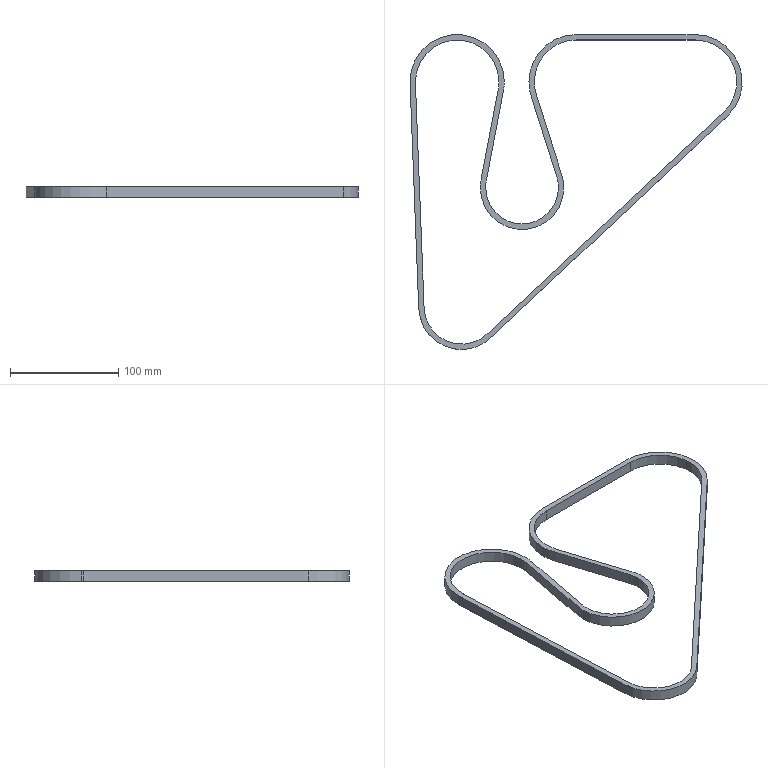Part | SolidWorks | features BeltProfileFeature 1, ExtruThin 1 | 1 solid | 32 faces | box 307.239 x 291.218 x 10 mm | volume 65563 mm3 | cylinder 20 | plane 12 | commonest cylinder face diameters 77.239 x9 87.239 x6 67.239 x3 69.196 x1 79.196 x1
STEP:
#1=CARTESIAN_POINT('',(33.941,200.791,10.));
#2=VERTEX_POINT('',#1);
#3=CARTESIAN_POINT('',(34.62,208.,10.));
#4=VERTEX_POINT('',#3);
#5=CARTESIAN_POINT('',(-4.,208.,10.));
#6=DIRECTION('',(0.,0.,1.));
#7=DIRECTION('',(-1.,0.,0.));
#8=AXIS2_PLACEMENT_3D('',#5,#6,#7);
#9=CIRCLE('',#8,38.62);
#10=EDGE_CURVE('',#2,#4,#9,.T.);
#11=ORIENTED_EDGE('',*,*,#10,.T.);
#12=CARTESIAN_POINT('',(34.62,208.,0.));
#13=VERTEX_POINT('',#12);
#14=CARTESIAN_POINT('',(34.62,208.,10.));
#15=DIRECTION('',(0.,0.,-1.));
#16=VECTOR('',#15,1000.);
#17=LINE('',#14,#16);
#18=EDGE_CURVE('',#4,#13,#17,.T.);
#19=ORIENTED_EDGE('',*,*,#18,.T.);
#20=CARTESIAN_POINT('',(33.941,200.791,0.));
#21=VERTEX_POINT('',#20);
#22=CARTESIAN_POINT('',(-4.,208.,0.));
#23=DIRECTION('',(0.,0.,1.));
#24=DIRECTION('',(-1.,0.,0.));
#25=AXIS2_PLACEMENT_3D('',#22,#23,#24);
#26=CIRCLE('',#25,38.62);
#27=EDGE_CURVE('',#21,#13,#26,.T.);
#28=ORIENTED_EDGE('',*,*,#27,.F.);
#29=CARTESIAN_POINT('',(33.941,200.791,10.));
#30=DIRECTION('',(0.,0.,-1.));
#31=VECTOR('',#30,1000.);
#32=LINE('',#29,#31);
#33=EDGE_CURVE('',#2,#21,#32,.T.);
#34=ORIENTED_EDGE('',*,*,#33,.F.);
#35=EDGE_LOOP('',(#11,#19,#28,#34));
#36=FACE_OUTER_BOUND('',#35,.T.);
#37=CARTESIAN_POINT('',(-4.,208.,10.));
#38=DIRECTION('',(0.,0.,-1.));
#39=DIRECTION('',(-1.,0.,0.));
#40=AXIS2_PLACEMENT_3D('',#37,#38,#39);
#41=CYLINDRICAL_SURFACE('',#40,38.62);
#42=ADVANCED_FACE('',(#36),#41,.F.);
#43=ORIENTED_EDGE('',*,*,#18,.F.);
#44=CARTESIAN_POINT('',(-42.62,208.,10.));
#45=VERTEX_POINT('',#44);
#46=CARTESIAN_POINT('',(-4.,208.,10.));
#47=DIRECTION('',(0.,0.,1.));
#48=DIRECTION('',(-1.,0.,0.));
#49=AXIS2_PLACEMENT_3D('',#46,#47,#48);
#50=CIRCLE('',#49,38.62);
#51=EDGE_CURVE('',#4,#45,#50,.T.);
#52=ORIENTED_EDGE('',*,*,#51,.T.);
#53=CARTESIAN_POINT('',(-42.62,208.,0.));
#54=VERTEX_POINT('',#53);
#55=CARTESIAN_POINT('',(-42.62,208.,10.));
#56=DIRECTION('',(0.,0.,-1.));
#57=VECTOR('',#56,1000.);
#58=LINE('',#55,#57);
#59=EDGE_CURVE('',#45,#54,#58,.T.);
#60=ORIENTED_EDGE('',*,*,#59,.T.);
#61=CARTESIAN_POINT('',(-4.,208.,0.));
#62=DIRECTION('',(0.,0.,1.));
#63=DIRECTION('',(-1.,0.,0.));
#64=AXIS2_PLACEMENT_3D('',#61,#62,#63);
#65=CIRCLE('',#64,38.62);
#66=EDGE_CURVE('',#13,#54,#65,.T.);
#67=ORIENTED_EDGE('',*,*,#66,.F.);
#68=EDGE_LOOP('',(#43,#52,#60,#67));
#69=FACE_OUTER_BOUND('',#68,.T.);
#70=CARTESIAN_POINT('',(-4.,208.,10.));
#71=DIRECTION('',(0.,0.,-1.));
#72=DIRECTION('',(-1.,0.,0.));
#73=AXIS2_PLACEMENT_3D('',#70,#71,#72);
#74=CYLINDRICAL_SURFACE('',#73,38.62);
#75=ADVANCED_FACE('',(#69),#74,.F.);
#76=CARTESIAN_POINT('',(92.82,121.653,10.));
#77=VERTEX_POINT('',#76);
#78=CARTESIAN_POINT('',(94.62,110.,10.));
#79=VERTEX_POINT('',#78);
#80=CARTESIAN_POINT('',(56.,110.,10.));
#81=DIRECTION('',(0.,0.,-1.));
#82=DIRECTION('',(1.,0.,0.));
#83=AXIS2_PLACEMENT_3D('',#80,#81,#82);
#84=CIRCLE('',#83,38.62);
#85=EDGE_CURVE('',#77,#79,#84,.T.);
#86=ORIENTED_EDGE('',*,*,#85,.T.);
#87=CARTESIAN_POINT('',(94.62,110.,0.));
#88=VERTEX_POINT('',#87);
#89=CARTESIAN_POINT('',(94.62,110.,10.));
#90=DIRECTION('',(0.,0.,-1.));
#91=VECTOR('',#90,1000.);
#92=LINE('',#89,#91);
#93=EDGE_CURVE('',#79,#88,#92,.T.);
#94=ORIENTED_EDGE('',*,*,#93,.T.);
#95=CARTESIAN_POINT('',(92.82,121.653,0.));
#96=VERTEX_POINT('',#95);
#97=CARTESIAN_POINT('',(56.,110.,0.));
#98=DIRECTION('',(0.,0.,-1.));
#99=DIRECTION('',(1.,0.,0.));
#100=AXIS2_PLACEMENT_3D('',#97,#98,#99);
#101=CIRCLE('',#100,38.62);
#102=EDGE_CURVE('',#96,#88,#101,.T.);
#103=ORIENTED_EDGE('',*,*,#102,.F.);
#104=CARTESIAN_POINT('',(92.82,121.653,10.));
#105=DIRECTION('',(0.,0.,-1.));
#106=VECTOR('',#105,1000.);
#107=LINE('',#104,#106);
#108=EDGE_CURVE('',#77,#96,#107,.T.);
#109=ORIENTED_EDGE('',*,*,#108,.F.);
#110=EDGE_LOOP('',(#86,#94,#103,#109));
#111=FACE_OUTER_BOUND('',#110,.T.);
#112=CARTESIAN_POINT('',(56.,110.,10.));
#113=DIRECTION('',(0.,0.,-1.));
#114=DIRECTION('',(-1.,0.,0.));
#115=AXIS2_PLACEMENT_3D('',#112,#113,#114);
#116=CYLINDRICAL_SURFACE('',#115,38.62);
#117=ADVANCED_FACE('',(#111),#116,.T.);
#118=ORIENTED_EDGE('',*,*,#93,.F.);
#119=CARTESIAN_POINT('',(17.38,110.,10.));
#120=VERTEX_POINT('',#119);
#121=CARTESIAN_POINT('',(56.,110.,10.));
#122=DIRECTION('',(0.,0.,-1.));
#123=DIRECTION('',(1.,0.,0.));
#124=AXIS2_PLACEMENT_3D('',#121,#122,#123);
#125=CIRCLE('',#124,38.62);
#126=EDGE_CURVE('',#79,#120,#125,.T.);
#127=ORIENTED_EDGE('',*,*,#126,.T.);
#128=CARTESIAN_POINT('',(17.38,110.,0.));
#129=VERTEX_POINT('',#128);
#130=CARTESIAN_POINT('',(17.38,110.,10.));
#131=DIRECTION('',(0.,0.,-1.));
#132=VECTOR('',#131,1000.);
#133=LINE('',#130,#132);
#134=EDGE_CURVE('',#120,#129,#133,.T.);
#135=ORIENTED_EDGE('',*,*,#134,.T.);
#136=CARTESIAN_POINT('',(56.,110.,0.));
#137=DIRECTION('',(0.,0.,-1.));
#138=DIRECTION('',(1.,0.,0.));
#139=AXIS2_PLACEMENT_3D('',#136,#137,#138);
#140=CIRCLE('',#139,38.62);
#141=EDGE_CURVE('',#88,#129,#140,.T.);
#142=ORIENTED_EDGE('',*,*,#141,.F.);
#143=EDGE_LOOP('',(#118,#127,#135,#142));
#144=FACE_OUTER_BOUND('',#143,.T.);
#145=CARTESIAN_POINT('',(56.,110.,10.));
#146=DIRECTION('',(0.,0.,-1.));
#147=DIRECTION('',(-1.,0.,0.));
#148=AXIS2_PLACEMENT_3D('',#145,#146,#147);
#149=CYLINDRICAL_SURFACE('',#148,38.62);
#150=ADVANCED_FACE('',(#144),#149,.T.);
#151=CARTESIAN_POINT('',(106.,246.62,10.));
#152=VERTEX_POINT('',#151);
#153=CARTESIAN_POINT('',(67.38,208.,10.));
#154=VERTEX_POINT('',#153);
#155=CARTESIAN_POINT('',(106.,208.,10.));
#156=DIRECTION('',(0.,0.,1.));
#157=DIRECTION('',(-1.,0.,0.));
#158=AXIS2_PLACEMENT_3D('',#155,#156,#157);
#159=CIRCLE('',#158,38.62);
#160=EDGE_CURVE('',#152,#154,#159,.T.);
#161=ORIENTED_EDGE('',*,*,#160,.T.);
#162=CARTESIAN_POINT('',(67.38,208.,0.));
#163=VERTEX_POINT('',#162);
#164=CARTESIAN_POINT('',(67.38,208.,10.));
#165=DIRECTION('',(0.,0.,-1.));
#166=VECTOR('',#165,1000.);
#167=LINE('',#164,#166);
#168=EDGE_CURVE('',#154,#163,#167,.T.);
#169=ORIENTED_EDGE('',*,*,#168,.T.);
#170=CARTESIAN_POINT('',(106.,246.62,0.));
#171=VERTEX_POINT('',#170);
#172=CARTESIAN_POINT('',(106.,208.,0.));
#173=DIRECTION('',(0.,0.,1.));
#174=DIRECTION('',(-1.,0.,0.));
#175=AXIS2_PLACEMENT_3D('',#172,#173,#174);
#176=CIRCLE('',#175,38.62);
#177=EDGE_CURVE('',#171,#163,#176,.T.);
#178=ORIENTED_EDGE('',*,*,#177,.F.);
#179=CARTESIAN_POINT('',(106.,246.62,10.));
#180=DIRECTION('',(0.,0.,-1.));
#181=VECTOR('',#180,1000.);
#182=LINE('',#179,#181);
#183=EDGE_CURVE('',#152,#171,#182,.T.);
#184=ORIENTED_EDGE('',*,*,#183,.F.);
#185=EDGE_LOOP('',(#161,#169,#178,#184));
#186=FACE_OUTER_BOUND('',#185,.T.);
#187=CARTESIAN_POINT('',(106.,208.,10.));
#188=DIRECTION('',(0.,0.,-1.));
#189=DIRECTION('',(-1.,0.,0.));
#190=AXIS2_PLACEMENT_3D('',#187,#188,#189);
#191=CYLINDRICAL_SURFACE('',#190,38.62);
#192=ADVANCED_FACE('',(#186),#191,.F.);
#193=CARTESIAN_POINT('',(39.62,208.,10.));
#194=VERTEX_POINT('',#193);
#195=CARTESIAN_POINT('',(-47.62,208.,10.));
#196=VERTEX_POINT('',#195);
#197=CARTESIAN_POINT('',(-4.,208.,10.));
#198=DIRECTION('',(0.,0.,1.));
#199=DIRECTION('',(-1.,0.,0.));
#200=AXIS2_PLACEMENT_3D('',#197,#198,#199);
#201=CIRCLE('',#200,43.62);
#202=EDGE_CURVE('',#194,#196,#201,.T.);
#203=ORIENTED_EDGE('',*,*,#202,.F.);
#204=CARTESIAN_POINT('',(39.62,208.,0.));
#205=VERTEX_POINT('',#204);
#206=CARTESIAN_POINT('',(39.62,208.,10.));
#207=DIRECTION('',(0.,0.,-1.));
#208=VECTOR('',#207,1000.);
#209=LINE('',#206,#208);
#210=EDGE_CURVE('',#194,#205,#209,.T.);
#211=ORIENTED_EDGE('',*,*,#210,.T.);
#212=CARTESIAN_POINT('',(-47.62,208.,0.));
#213=VERTEX_POINT('',#212);
#214=CARTESIAN_POINT('',(-4.,208.,0.));
#215=DIRECTION('',(0.,0.,1.));
#216=DIRECTION('',(-1.,0.,0.));
#217=AXIS2_PLACEMENT_3D('',#214,#215,#216);
#218=CIRCLE('',#217,43.62);
#219=EDGE_CURVE('',#205,#213,#218,.T.);
#220=ORIENTED_EDGE('',*,*,#219,.T.);
#221=CARTESIAN_POINT('',(-47.62,208.,10.));
#222=DIRECTION('',(0.,0.,-1.));
#223=VECTOR('',#222,1000.);
#224=LINE('',#221,#223);
#225=EDGE_CURVE('',#196,#213,#224,.T.);
#226=ORIENTED_EDGE('',*,*,#225,.F.);
#227=EDGE_LOOP('',(#203,#211,#220,#226));
#228=FACE_OUTER_BOUND('',#227,.T.);
#229=CARTESIAN_POINT('',(-4.,208.,10.));
#230=DIRECTION('',(0.,0.,-1.));
#231=DIRECTION('',(-1.,0.,0.));
#232=AXIS2_PLACEMENT_3D('',#229,#230,#231);
#233=CYLINDRICAL_SURFACE('',#232,43.62);
#234=ADVANCED_FACE('',(#228),#233,.T.);
#235=CARTESIAN_POINT('',(-47.587,206.318,10.));
#236=VERTEX_POINT('',#235);
#237=CARTESIAN_POINT('',(-4.,208.,10.));
#238=DIRECTION('',(0.,0.,1.));
#239=DIRECTION('',(-1.,0.,0.));
#240=AXIS2_PLACEMENT_3D('',#237,#238,#239);
#241=CIRCLE('',#240,43.62);
#242=EDGE_CURVE('',#196,#236,#241,.T.);
#243=ORIENTED_EDGE('',*,*,#242,.F.);
#244=ORIENTED_EDGE('',*,*,#225,.T.);
#245=CARTESIAN_POINT('',(-47.587,206.318,0.));
#246=VERTEX_POINT('',#245);
#247=CARTESIAN_POINT('',(-4.,208.,0.));
#248=DIRECTION('',(0.,0.,1.));
#249=DIRECTION('',(-1.,0.,0.));
#250=AXIS2_PLACEMENT_3D('',#247,#248,#249);
#251=CIRCLE('',#250,43.62);
#252=EDGE_CURVE('',#213,#246,#251,.T.);
#253=ORIENTED_EDGE('',*,*,#252,.T.);
#254=CARTESIAN_POINT('',(-47.587,206.318,10.));
#255=DIRECTION('',(0.,0.,-1.));
#256=VECTOR('',#255,1000.);
#257=LINE('',#254,#256);
#258=EDGE_CURVE('',#236,#246,#257,.T.);
#259=ORIENTED_EDGE('',*,*,#258,.F.);
#260=EDGE_LOOP('',(#243,#244,#253,#259));
#261=FACE_OUTER_BOUND('',#260,.T.);
#262=CARTESIAN_POINT('',(-4.,208.,10.));
#263=DIRECTION('',(0.,0.,-1.));
#264=DIRECTION('',(-1.,0.,0.));
#265=AXIS2_PLACEMENT_3D('',#262,#263,#264);
#266=CYLINDRICAL_SURFACE('',#265,43.62);
#267=ADVANCED_FACE('',(#261),#266,.T.);
#268=CARTESIAN_POINT('',(89.62,110.,10.));
#269=VERTEX_POINT('',#268);
#270=CARTESIAN_POINT('',(22.38,110.,10.));
#271=VERTEX_POINT('',#270);
#272=CARTESIAN_POINT('',(56.,110.,10.));
#273=DIRECTION('',(0.,0.,-1.));
#274=DIRECTION('',(-1.,0.,0.));
#275=AXIS2_PLACEMENT_3D('',#272,#273,#274);
#276=CIRCLE('',#275,33.62);
#277=EDGE_CURVE('',#269,#271,#276,.T.);
#278=ORIENTED_EDGE('',*,*,#277,.F.);
#279=CARTESIAN_POINT('',(89.62,110.,0.));
#280=VERTEX_POINT('',#279);
#281=CARTESIAN_POINT('',(89.62,110.,10.));
#282=DIRECTION('',(0.,0.,-1.));
#283=VECTOR('',#282,1000.);
#284=LINE('',#281,#283);
#285=EDGE_CURVE('',#269,#280,#284,.T.);
#286=ORIENTED_EDGE('',*,*,#285,.T.);
#287=CARTESIAN_POINT('',(22.38,110.,0.));
#288=VERTEX_POINT('',#287);
#289=CARTESIAN_POINT('',(56.,110.,0.));
#290=DIRECTION('',(0.,0.,-1.));
#291=DIRECTION('',(-1.,0.,0.));
#292=AXIS2_PLACEMENT_3D('',#289,#290,#291);
#293=CIRCLE('',#292,33.62);
#294=EDGE_CURVE('',#280,#288,#293,.T.);
#295=ORIENTED_EDGE('',*,*,#294,.T.);
#296=CARTESIAN_POINT('',(22.38,110.,10.));
#297=DIRECTION('',(0.,0.,-1.));
#298=VECTOR('',#297,1000.);
#299=LINE('',#296,#298);
#300=EDGE_CURVE('',#271,#288,#299,.T.);
#301=ORIENTED_EDGE('',*,*,#300,.F.);
#302=EDGE_LOOP('',(#278,#286,#295,#301));
#303=FACE_OUTER_BOUND('',#302,.T.);
#304=CARTESIAN_POINT('',(56.,110.,10.));
#305=DIRECTION('',(0.,0.,-1.));
#306=DIRECTION('',(-1.,0.,0.));
#307=AXIS2_PLACEMENT_3D('',#304,#305,#306);
#308=CYLINDRICAL_SURFACE('',#307,33.62);
#309=ADVANCED_FACE('',(#303),#308,.F.);
#310=CARTESIAN_POINT('',(22.971,116.276,10.));
#311=VERTEX_POINT('',#310);
#312=CARTESIAN_POINT('',(56.,110.,10.));
#313=DIRECTION('',(0.,0.,-1.));
#314=DIRECTION('',(-1.,0.,0.));
#315=AXIS2_PLACEMENT_3D('',#312,#313,#314);
#316=CIRCLE('',#315,33.62);
#317=EDGE_CURVE('',#271,#311,#316,.T.);
#318=ORIENTED_EDGE('',*,*,#317,.F.);
#319=ORIENTED_EDGE('',*,*,#300,.T.);
#320=CARTESIAN_POINT('',(22.971,116.276,0.));
#321=VERTEX_POINT('',#320);
#322=CARTESIAN_POINT('',(56.,110.,0.));
#323=DIRECTION('',(0.,0.,-1.));
#324=DIRECTION('',(-1.,0.,0.));
#325=AXIS2_PLACEMENT_3D('',#322,#323,#324);
#326=CIRCLE('',#325,33.62);
#327=EDGE_CURVE('',#288,#321,#326,.T.);
#328=ORIENTED_EDGE('',*,*,#327,.T.);
#329=CARTESIAN_POINT('',(22.971,116.276,10.));
#330=DIRECTION('',(0.,0.,-1.));
#331=VECTOR('',#330,1000.);
#332=LINE('',#329,#331);
#333=EDGE_CURVE('',#311,#321,#332,.T.);
#334=ORIENTED_EDGE('',*,*,#333,.F.);
#335=EDGE_LOOP('',(#318,#319,#328,#334));
#336=FACE_OUTER_BOUND('',#335,.T.);
#337=CARTESIAN_POINT('',(56.,110.,10.));
#338=DIRECTION('',(0.,0.,-1.));
#339=DIRECTION('',(-1.,0.,0.));
#340=AXIS2_PLACEMENT_3D('',#337,#338,#339);
#341=CYLINDRICAL_SURFACE('',#340,33.62);
#342=ADVANCED_FACE('',(#336),#341,.F.);
#343=CARTESIAN_POINT('',(62.38,208.,10.));
#344=VERTEX_POINT('',#343);
#345=CARTESIAN_POINT('',(64.413,194.839,10.));
#346=VERTEX_POINT('',#345);
#347=CARTESIAN_POINT('',(106.,208.,10.));
#348=DIRECTION('',(0.,0.,1.));
#349=DIRECTION('',(-1.,0.,0.));
#350=AXIS2_PLACEMENT_3D('',#347,#348,#349);
#351=CIRCLE('',#350,43.62);
#352=EDGE_CURVE('',#344,#346,#351,.T.);
#353=ORIENTED_EDGE('',*,*,#352,.F.);
#354=CARTESIAN_POINT('',(62.38,208.,0.));
#355=VERTEX_POINT('',#354);
#356=CARTESIAN_POINT('',(62.38,208.,10.));
#357=DIRECTION('',(0.,0.,-1.));
#358=VECTOR('',#357,1000.);
#359=LINE('',#356,#358);
#360=EDGE_CURVE('',#344,#355,#359,.T.);
#361=ORIENTED_EDGE('',*,*,#360,.T.);
#362=CARTESIAN_POINT('',(64.413,194.839,0.));
#363=VERTEX_POINT('',#362);
#364=CARTESIAN_POINT('',(106.,208.,0.));
#365=DIRECTION('',(0.,0.,1.));
#366=DIRECTION('',(-1.,0.,0.));
#367=AXIS2_PLACEMENT_3D('',#364,#365,#366);
#368=CIRCLE('',#367,43.62);
#369=EDGE_CURVE('',#355,#363,#368,.T.);
#370=ORIENTED_EDGE('',*,*,#369,.T.);
#371=CARTESIAN_POINT('',(64.413,194.839,10.));
#372=DIRECTION('',(0.,0.,-1.));
#373=VECTOR('',#372,1000.);
#374=LINE('',#371,#373);
#375=EDGE_CURVE('',#346,#363,#374,.T.);
#376=ORIENTED_EDGE('',*,*,#375,.F.);
#377=EDGE_LOOP('',(#353,#361,#370,#376));
#378=FACE_OUTER_BOUND('',#377,.T.);
#379=CARTESIAN_POINT('',(106.,208.,10.));
#380=DIRECTION('',(0.,0.,-1.));
#381=DIRECTION('',(-1.,0.,0.));
#382=AXIS2_PLACEMENT_3D('',#379,#380,#381);
#383=CYLINDRICAL_SURFACE('',#382,43.62);
#384=ADVANCED_FACE('',(#378),#383,.T.);
#385=CARTESIAN_POINT('',(-39.568,-1.527,10.));
#386=VERTEX_POINT('',#385);
#387=CARTESIAN_POINT('',(27.082,-28.889,10.));
#388=VERTEX_POINT('',#387);
#389=CARTESIAN_POINT('',(0.,0.,10.));
#390=DIRECTION('',(0.,0.,1.));
#391=DIRECTION('',(-1.,0.,0.));
#392=AXIS2_PLACEMENT_3D('',#389,#390,#391);
#393=CIRCLE('',#392,39.598);
#394=EDGE_CURVE('',#386,#388,#393,.T.);
#395=ORIENTED_EDGE('',*,*,#394,.T.);
#396=CARTESIAN_POINT('',(245.832,176.177,10.));
#397=VERTEX_POINT('',#396);
#398=CARTESIAN_POINT('',(27.082,-28.889,10.));
#399=DIRECTION('',(0.7296,0.6839,0.));
#400=VECTOR('',#399,1000.);
#401=LINE('',#398,#400);
#402=EDGE_CURVE('',#388,#397,#401,.T.);
#403=ORIENTED_EDGE('',*,*,#402,.T.);
#404=CARTESIAN_POINT('',(216.,251.62,10.));
#405=VERTEX_POINT('',#404);
#406=CARTESIAN_POINT('',(216.,208.,10.));
#407=DIRECTION('',(0.,0.,1.));
#408=DIRECTION('',(-1.,0.,0.));
#409=AXIS2_PLACEMENT_3D('',#406,#407,#408);
#410=CIRCLE('',#409,43.62);
#411=EDGE_CURVE('',#397,#405,#410,.T.);
#412=ORIENTED_EDGE('',*,*,#411,.T.);
#413=CARTESIAN_POINT('',(106.,251.62,10.));
#414=VERTEX_POINT('',#413);
#415=CARTESIAN_POINT('',(0.,251.62,10.));
#416=DIRECTION('',(-1.,0.,0.));
#417=VECTOR('',#416,1000.);
#418=LINE('',#415,#417);
#419=EDGE_CURVE('',#405,#414,#418,.T.);
#420=ORIENTED_EDGE('',*,*,#419,.T.);
#421=CARTESIAN_POINT('',(106.,208.,10.));
#422=DIRECTION('',(0.,0.,1.));
#423=DIRECTION('',(-1.,0.,0.));
#424=AXIS2_PLACEMENT_3D('',#421,#422,#423);
#425=CIRCLE('',#424,43.62);
#426=EDGE_CURVE('',#414,#344,#425,.T.);
#427=ORIENTED_EDGE('',*,*,#426,.T.);
#428=ORIENTED_EDGE('',*,*,#352,.T.);
#429=CARTESIAN_POINT('',(88.053,120.144,10.));
#430=VERTEX_POINT('',#429);
#431=CARTESIAN_POINT('',(114.598,36.268,10.));
#432=DIRECTION('',(0.3017,-0.9534,0.));
#433=VECTOR('',#432,1000.);
#434=LINE('',#431,#433);
#435=EDGE_CURVE('',#346,#430,#434,.T.);
#436=ORIENTED_EDGE('',*,*,#435,.T.);
#437=CARTESIAN_POINT('',(56.,110.,10.));
#438=DIRECTION('',(0.,0.,-1.));
#439=DIRECTION('',(-1.,0.,0.));
#440=AXIS2_PLACEMENT_3D('',#437,#438,#439);
#441=CIRCLE('',#440,33.62);
#442=EDGE_CURVE('',#430,#269,#441,.T.);
#443=ORIENTED_EDGE('',*,*,#442,.T.);
#444=ORIENTED_EDGE('',*,*,#277,.T.);
#445=ORIENTED_EDGE('',*,*,#317,.T.);
#446=CARTESIAN_POINT('',(38.853,199.857,10.));
#447=VERTEX_POINT('',#446);
#448=CARTESIAN_POINT('',(0.8468,-0.1609,10.));
#449=DIRECTION('',(0.1867,0.9824,0.));
#450=VECTOR('',#449,1000.);
#451=LINE('',#448,#450);
#452=EDGE_CURVE('',#311,#447,#451,.T.);
#453=ORIENTED_EDGE('',*,*,#452,.T.);
#454=CARTESIAN_POINT('',(-4.,208.,10.));
#455=DIRECTION('',(0.,0.,1.));
#456=DIRECTION('',(-1.,0.,0.));
#457=AXIS2_PLACEMENT_3D('',#454,#455,#456);
#458=CIRCLE('',#457,43.62);
#459=EDGE_CURVE('',#447,#194,#458,.T.);
#460=ORIENTED_EDGE('',*,*,#459,.T.);
#461=ORIENTED_EDGE('',*,*,#202,.T.);
#462=ORIENTED_EDGE('',*,*,#242,.T.);
#463=CARTESIAN_POINT('',(-39.568,-1.527,10.));
#464=DIRECTION('',(0.03855,-0.9993,0.));
#465=VECTOR('',#464,1000.);
#466=LINE('',#463,#465);
#467=EDGE_CURVE('',#236,#386,#466,.T.);
#468=ORIENTED_EDGE('',*,*,#467,.T.);
#469=EDGE_LOOP('',(#395,#403,#412,#420,#427,#428,#436,#443,#444,#445,#453,#460,#461,#462,#468));
#470=FACE_OUTER_BOUND('',#469,.T.);
#471=CARTESIAN_POINT('',(-34.572,-1.334,10.));
#472=VERTEX_POINT('',#471);
#473=CARTESIAN_POINT('',(23.662,-25.241,10.));
#474=VERTEX_POINT('',#473);
#475=CARTESIAN_POINT('',(0.,0.,10.));
#476=DIRECTION('',(0.,0.,1.));
#477=DIRECTION('',(-1.,0.,0.));
#478=AXIS2_PLACEMENT_3D('',#475,#476,#477);
#479=CIRCLE('',#478,34.598);
#480=EDGE_CURVE('',#472,#474,#479,.T.);
#481=ORIENTED_EDGE('',*,*,#480,.F.);
#482=CARTESIAN_POINT('',(-42.591,206.511,10.));
#483=VERTEX_POINT('',#482);
#484=CARTESIAN_POINT('',(-34.572,-1.334,10.));
#485=DIRECTION('',(0.03855,-0.9993,0.));
#486=VECTOR('',#485,1000.);
#487=LINE('',#484,#486);
#488=EDGE_CURVE('',#483,#472,#487,.T.);
#489=ORIENTED_EDGE('',*,*,#488,.F.);
#490=CARTESIAN_POINT('',(-4.,208.,10.));
#491=DIRECTION('',(0.,0.,1.));
#492=DIRECTION('',(-1.,0.,0.));
#493=AXIS2_PLACEMENT_3D('',#490,#491,#492);
#494=CIRCLE('',#493,38.62);
#495=EDGE_CURVE('',#45,#483,#494,.T.);
#496=ORIENTED_EDGE('',*,*,#495,.F.);
#497=ORIENTED_EDGE('',*,*,#51,.F.);
#498=ORIENTED_EDGE('',*,*,#10,.F.);
#499=CARTESIAN_POINT('',(18.059,117.209,10.));
#500=VERTEX_POINT('',#499);
#501=CARTESIAN_POINT('',(33.941,200.791,10.));
#502=DIRECTION('',(0.1867,0.9824,0.));
#503=VECTOR('',#502,1000.);
#504=LINE('',#501,#503);
#505=EDGE_CURVE('',#500,#2,#504,.T.);
#506=ORIENTED_EDGE('',*,*,#505,.F.);
#507=CARTESIAN_POINT('',(56.,110.,10.));
#508=DIRECTION('',(0.,0.,-1.));
#509=DIRECTION('',(1.,0.,0.));
#510=AXIS2_PLACEMENT_3D('',#507,#508,#509);
#511=CIRCLE('',#510,38.62);
#512=EDGE_CURVE('',#120,#500,#511,.T.);
#513=ORIENTED_EDGE('',*,*,#512,.F.);
#514=ORIENTED_EDGE('',*,*,#126,.F.);
#515=ORIENTED_EDGE('',*,*,#85,.F.);
#516=CARTESIAN_POINT('',(69.18,196.347,10.));
#517=VERTEX_POINT('',#516);
#518=CARTESIAN_POINT('',(92.82,121.653,10.));
#519=DIRECTION('',(0.3017,-0.9534,0.));
#520=VECTOR('',#519,1000.);
#521=LINE('',#518,#520);
#522=EDGE_CURVE('',#517,#77,#521,.T.);
#523=ORIENTED_EDGE('',*,*,#522,.F.);
#524=CARTESIAN_POINT('',(106.,208.,10.));
#525=DIRECTION('',(0.,0.,1.));
#526=DIRECTION('',(-1.,0.,0.));
#527=AXIS2_PLACEMENT_3D('',#524,#525,#526);
#528=CIRCLE('',#527,38.62);
#529=EDGE_CURVE('',#154,#517,#528,.T.);
#530=ORIENTED_EDGE('',*,*,#529,.F.);
#531=ORIENTED_EDGE('',*,*,#160,.F.);
#532=CARTESIAN_POINT('',(216.,246.62,10.));
#533=VERTEX_POINT('',#532);
#534=CARTESIAN_POINT('',(106.,246.62,10.));
#535=DIRECTION('',(-1.,0.,0.));
#536=VECTOR('',#535,1000.);
#537=LINE('',#534,#536);
#538=EDGE_CURVE('',#533,#152,#537,.T.);
#539=ORIENTED_EDGE('',*,*,#538,.F.);
#540=CARTESIAN_POINT('',(242.413,179.825,10.));
#541=VERTEX_POINT('',#540);
#542=CARTESIAN_POINT('',(216.,208.,10.));
#543=DIRECTION('',(0.,0.,1.));
#544=DIRECTION('',(-1.,0.,0.));
#545=AXIS2_PLACEMENT_3D('',#542,#543,#544);
#546=CIRCLE('',#545,38.62);
#547=EDGE_CURVE('',#541,#533,#546,.T.);
#548=ORIENTED_EDGE('',*,*,#547,.F.);
#549=CARTESIAN_POINT('',(242.413,179.825,10.));
#550=DIRECTION('',(0.7296,0.6839,0.));
#551=VECTOR('',#550,1000.);
#552=LINE('',#549,#551);
#553=EDGE_CURVE('',#474,#541,#552,.T.);
#554=ORIENTED_EDGE('',*,*,#553,.F.);
#555=EDGE_LOOP('',(#481,#489,#496,#497,#498,#506,#513,#514,#515,#523,#530,#531,#539,#548,#554));
#556=FACE_BOUND('',#555,.T.);
#557=CARTESIAN_POINT('',(0.,0.,10.));
#558=DIRECTION('',(0.,0.,-1.));
#559=DIRECTION('',(-1.,0.,0.));
#560=AXIS2_PLACEMENT_3D('',#557,#558,#559);
#561=PLANE('',#560);
#562=ADVANCED_FACE('',(#470,#556),#561,.F.);
#563=CARTESIAN_POINT('',(-39.568,-1.527,0.));
#564=VERTEX_POINT('',#563);
#565=CARTESIAN_POINT('',(27.082,-28.889,0.));
#566=VERTEX_POINT('',#565);
#567=CARTESIAN_POINT('',(0.,0.,0.));
#568=DIRECTION('',(0.,0.,1.));
#569=DIRECTION('',(-1.,0.,0.));
#570=AXIS2_PLACEMENT_3D('',#567,#568,#569);
#571=CIRCLE('',#570,39.598);
#572=EDGE_CURVE('',#564,#566,#571,.T.);
#573=ORIENTED_EDGE('',*,*,#572,.F.);
#574=CARTESIAN_POINT('',(-39.568,-1.527,0.));
#575=DIRECTION('',(0.03855,-0.9993,0.));
#576=VECTOR('',#575,1000.);
#577=LINE('',#574,#576);
#578=EDGE_CURVE('',#246,#564,#577,.T.);
#579=ORIENTED_EDGE('',*,*,#578,.F.);
#580=ORIENTED_EDGE('',*,*,#252,.F.);
#581=ORIENTED_EDGE('',*,*,#219,.F.);
#582=CARTESIAN_POINT('',(38.853,199.857,0.));
#583=VERTEX_POINT('',#582);
#584=CARTESIAN_POINT('',(-4.,208.,0.));
#585=DIRECTION('',(0.,0.,1.));
#586=DIRECTION('',(-1.,0.,0.));
#587=AXIS2_PLACEMENT_3D('',#584,#585,#586);
#588=CIRCLE('',#587,43.62);
#589=EDGE_CURVE('',#583,#205,#588,.T.);
#590=ORIENTED_EDGE('',*,*,#589,.F.);
#591=CARTESIAN_POINT('',(0.8468,-0.1609,0.));
#592=DIRECTION('',(0.1867,0.9824,0.));
#593=VECTOR('',#592,1000.);
#594=LINE('',#591,#593);
#595=EDGE_CURVE('',#321,#583,#594,.T.);
#596=ORIENTED_EDGE('',*,*,#595,.F.);
#597=ORIENTED_EDGE('',*,*,#327,.F.);
#598=ORIENTED_EDGE('',*,*,#294,.F.);
#599=CARTESIAN_POINT('',(88.053,120.144,0.));
#600=VERTEX_POINT('',#599);
#601=CARTESIAN_POINT('',(56.,110.,0.));
#602=DIRECTION('',(0.,0.,-1.));
#603=DIRECTION('',(-1.,0.,0.));
#604=AXIS2_PLACEMENT_3D('',#601,#602,#603);
#605=CIRCLE('',#604,33.62);
#606=EDGE_CURVE('',#600,#280,#605,.T.);
#607=ORIENTED_EDGE('',*,*,#606,.F.);
#608=CARTESIAN_POINT('',(114.598,36.268,0.));
#609=DIRECTION('',(0.3017,-0.9534,0.));
#610=VECTOR('',#609,1000.);
#611=LINE('',#608,#610);
#612=EDGE_CURVE('',#363,#600,#611,.T.);
#613=ORIENTED_EDGE('',*,*,#612,.F.);
#614=ORIENTED_EDGE('',*,*,#369,.F.);
#615=CARTESIAN_POINT('',(106.,251.62,0.));
#616=VERTEX_POINT('',#615);
#617=CARTESIAN_POINT('',(106.,208.,0.));
#618=DIRECTION('',(0.,0.,1.));
#619=DIRECTION('',(-1.,0.,0.));
#620=AXIS2_PLACEMENT_3D('',#617,#618,#619);
#621=CIRCLE('',#620,43.62);
#622=EDGE_CURVE('',#616,#355,#621,.T.);
#623=ORIENTED_EDGE('',*,*,#622,.F.);
#624=CARTESIAN_POINT('',(216.,251.62,0.));
#625=VERTEX_POINT('',#624);
#626=CARTESIAN_POINT('',(0.,251.62,0.));
#627=DIRECTION('',(-1.,0.,0.));
#628=VECTOR('',#627,1000.);
#629=LINE('',#626,#628);
#630=EDGE_CURVE('',#625,#616,#629,.T.);
#631=ORIENTED_EDGE('',*,*,#630,.F.);
#632=CARTESIAN_POINT('',(245.832,176.177,0.));
#633=VERTEX_POINT('',#632);
#634=CARTESIAN_POINT('',(216.,208.,0.));
#635=DIRECTION('',(0.,0.,1.));
#636=DIRECTION('',(-1.,0.,0.));
#637=AXIS2_PLACEMENT_3D('',#634,#635,#636);
#638=CIRCLE('',#637,43.62);
#639=EDGE_CURVE('',#633,#625,#638,.T.);
#640=ORIENTED_EDGE('',*,*,#639,.F.);
#641=CARTESIAN_POINT('',(27.082,-28.889,0.));
#642=DIRECTION('',(0.7296,0.6839,0.));
#643=VECTOR('',#642,1000.);
#644=LINE('',#641,#643);
#645=EDGE_CURVE('',#566,#633,#644,.T.);
#646=ORIENTED_EDGE('',*,*,#645,.F.);
#647=EDGE_LOOP('',(#573,#579,#580,#581,#590,#596,#597,#598,#607,#613,#614,#623,#631,#640,#646));
#648=FACE_OUTER_BOUND('',#647,.T.);
#649=CARTESIAN_POINT('',(-42.591,206.511,0.));
#650=VERTEX_POINT('',#649);
#651=CARTESIAN_POINT('',(-34.572,-1.334,0.));
#652=VERTEX_POINT('',#651);
#653=CARTESIAN_POINT('',(-34.572,-1.334,0.));
#654=DIRECTION('',(0.03855,-0.9993,0.));
#655=VECTOR('',#654,1000.);
#656=LINE('',#653,#655);
#657=EDGE_CURVE('',#650,#652,#656,.T.);
#658=ORIENTED_EDGE('',*,*,#657,.T.);
#659=CARTESIAN_POINT('',(23.662,-25.241,0.));
#660=VERTEX_POINT('',#659);
#661=CARTESIAN_POINT('',(0.,0.,0.));
#662=DIRECTION('',(0.,0.,1.));
#663=DIRECTION('',(-1.,0.,0.));
#664=AXIS2_PLACEMENT_3D('',#661,#662,#663);
#665=CIRCLE('',#664,34.598);
#666=EDGE_CURVE('',#652,#660,#665,.T.);
#667=ORIENTED_EDGE('',*,*,#666,.T.);
#668=CARTESIAN_POINT('',(242.413,179.825,0.));
#669=VERTEX_POINT('',#668);
#670=CARTESIAN_POINT('',(242.413,179.825,0.));
#671=DIRECTION('',(0.7296,0.6839,0.));
#672=VECTOR('',#671,1000.);
#673=LINE('',#670,#672);
#674=EDGE_CURVE('',#660,#669,#673,.T.);
#675=ORIENTED_EDGE('',*,*,#674,.T.);
#676=CARTESIAN_POINT('',(216.,246.62,0.));
#677=VERTEX_POINT('',#676);
#678=CARTESIAN_POINT('',(216.,208.,0.));
#679=DIRECTION('',(0.,0.,1.));
#680=DIRECTION('',(-1.,0.,0.));
#681=AXIS2_PLACEMENT_3D('',#678,#679,#680);
#682=CIRCLE('',#681,38.62);
#683=EDGE_CURVE('',#669,#677,#682,.T.);
#684=ORIENTED_EDGE('',*,*,#683,.T.);
#685=CARTESIAN_POINT('',(106.,246.62,0.));
#686=DIRECTION('',(-1.,0.,0.));
#687=VECTOR('',#686,1000.);
#688=LINE('',#685,#687);
#689=EDGE_CURVE('',#677,#171,#688,.T.);
#690=ORIENTED_EDGE('',*,*,#689,.T.);
#691=ORIENTED_EDGE('',*,*,#177,.T.);
#692=CARTESIAN_POINT('',(69.18,196.347,0.));
#693=VERTEX_POINT('',#692);
#694=CARTESIAN_POINT('',(106.,208.,0.));
#695=DIRECTION('',(0.,0.,1.));
#696=DIRECTION('',(-1.,0.,0.));
#697=AXIS2_PLACEMENT_3D('',#694,#695,#696);
#698=CIRCLE('',#697,38.62);
#699=EDGE_CURVE('',#163,#693,#698,.T.);
#700=ORIENTED_EDGE('',*,*,#699,.T.);
#701=CARTESIAN_POINT('',(92.82,121.653,0.));
#702=DIRECTION('',(0.3017,-0.9534,0.));
#703=VECTOR('',#702,1000.);
#704=LINE('',#701,#703);
#705=EDGE_CURVE('',#693,#96,#704,.T.);
#706=ORIENTED_EDGE('',*,*,#705,.T.);
#707=ORIENTED_EDGE('',*,*,#102,.T.);
#708=ORIENTED_EDGE('',*,*,#141,.T.);
#709=CARTESIAN_POINT('',(18.059,117.209,0.));
#710=VERTEX_POINT('',#709);
#711=CARTESIAN_POINT('',(56.,110.,0.));
#712=DIRECTION('',(0.,0.,-1.));
#713=DIRECTION('',(1.,0.,0.));
#714=AXIS2_PLACEMENT_3D('',#711,#712,#713);
#715=CIRCLE('',#714,38.62);
#716=EDGE_CURVE('',#129,#710,#715,.T.);
#717=ORIENTED_EDGE('',*,*,#716,.T.);
#718=CARTESIAN_POINT('',(33.941,200.791,0.));
#719=DIRECTION('',(0.1867,0.9824,0.));
#720=VECTOR('',#719,1000.);
#721=LINE('',#718,#720);
#722=EDGE_CURVE('',#710,#21,#721,.T.);
#723=ORIENTED_EDGE('',*,*,#722,.T.);
#724=ORIENTED_EDGE('',*,*,#27,.T.);
#725=ORIENTED_EDGE('',*,*,#66,.T.);
#726=CARTESIAN_POINT('',(-4.,208.,0.));
#727=DIRECTION('',(0.,0.,1.));
#728=DIRECTION('',(-1.,0.,0.));
#729=AXIS2_PLACEMENT_3D('',#726,#727,#728);
#730=CIRCLE('',#729,38.62);
#731=EDGE_CURVE('',#54,#650,#730,.T.);
#732=ORIENTED_EDGE('',*,*,#731,.T.);
#733=EDGE_LOOP('',(#658,#667,#675,#684,#690,#691,#700,#706,#707,#708,#717,#723,#724,#725,#732));
#734=FACE_BOUND('',#733,.T.);
#735=CARTESIAN_POINT('',(0.,0.,0.));
#736=DIRECTION('',(0.,0.,-1.));
#737=DIRECTION('',(-1.,0.,0.));
#738=AXIS2_PLACEMENT_3D('',#735,#736,#737);
#739=PLANE('',#738);
#740=ADVANCED_FACE('',(#648,#734),#739,.T.);
#741=ORIENTED_EDGE('',*,*,#572,.T.);
#742=CARTESIAN_POINT('',(27.082,-28.889,10.));
#743=DIRECTION('',(0.,0.,-1.));
#744=VECTOR('',#743,1000.);
#745=LINE('',#742,#744);
#746=EDGE_CURVE('',#388,#566,#745,.T.);
#747=ORIENTED_EDGE('',*,*,#746,.F.);
#748=ORIENTED_EDGE('',*,*,#394,.F.);
#749=CARTESIAN_POINT('',(-39.568,-1.527,10.));
#750=DIRECTION('',(0.,0.,-1.));
#751=VECTOR('',#750,1000.);
#752=LINE('',#749,#751);
#753=EDGE_CURVE('',#386,#564,#752,.T.);
#754=ORIENTED_EDGE('',*,*,#753,.T.);
#755=EDGE_LOOP('',(#741,#747,#748,#754));
#756=FACE_OUTER_BOUND('',#755,.T.);
#757=CARTESIAN_POINT('',(0.,0.,10.));
#758=DIRECTION('',(0.,0.,-1.));
#759=DIRECTION('',(-1.,0.,0.));
#760=AXIS2_PLACEMENT_3D('',#757,#758,#759);
#761=CYLINDRICAL_SURFACE('',#760,39.598);
#762=ADVANCED_FACE('',(#756),#761,.T.);
#763=ORIENTED_EDGE('',*,*,#645,.T.);
#764=CARTESIAN_POINT('',(245.832,176.177,10.));
#765=DIRECTION('',(0.,0.,-1.));
#766=VECTOR('',#765,1000.);
#767=LINE('',#764,#766);
#768=EDGE_CURVE('',#397,#633,#767,.T.);
#769=ORIENTED_EDGE('',*,*,#768,.F.);
#770=ORIENTED_EDGE('',*,*,#402,.F.);
#771=ORIENTED_EDGE('',*,*,#746,.T.);
#772=EDGE_LOOP('',(#763,#769,#770,#771));
#773=FACE_OUTER_BOUND('',#772,.T.);
#774=CARTESIAN_POINT('',(27.082,-28.889,10.));
#775=DIRECTION('',(-0.6839,0.7296,0.));
#776=DIRECTION('',(-0.7296,-0.6839,0.));
#777=AXIS2_PLACEMENT_3D('',#774,#775,#776);
#778=PLANE('',#777);
#779=ADVANCED_FACE('',(#773),#778,.F.);
#780=ORIENTED_EDGE('',*,*,#639,.T.);
#781=CARTESIAN_POINT('',(216.,251.62,10.));
#782=DIRECTION('',(0.,0.,-1.));
#783=VECTOR('',#782,1000.);
#784=LINE('',#781,#783);
#785=EDGE_CURVE('',#405,#625,#784,.T.);
#786=ORIENTED_EDGE('',*,*,#785,.F.);
#787=ORIENTED_EDGE('',*,*,#411,.F.);
#788=ORIENTED_EDGE('',*,*,#768,.T.);
#789=EDGE_LOOP('',(#780,#786,#787,#788));
#790=FACE_OUTER_BOUND('',#789,.T.);
#791=CARTESIAN_POINT('',(216.,208.,10.));
#792=DIRECTION('',(0.,0.,-1.));
#793=DIRECTION('',(-1.,0.,0.));
#794=AXIS2_PLACEMENT_3D('',#791,#792,#793);
#795=CYLINDRICAL_SURFACE('',#794,43.62);
#796=ADVANCED_FACE('',(#790),#795,.T.);
#797=ORIENTED_EDGE('',*,*,#630,.T.);
#798=CARTESIAN_POINT('',(106.,251.62,10.));
#799=DIRECTION('',(0.,0.,-1.));
#800=VECTOR('',#799,1000.);
#801=LINE('',#798,#800);
#802=EDGE_CURVE('',#414,#616,#801,.T.);
#803=ORIENTED_EDGE('',*,*,#802,.F.);
#804=ORIENTED_EDGE('',*,*,#419,.F.);
#805=ORIENTED_EDGE('',*,*,#785,.T.);
#806=EDGE_LOOP('',(#797,#803,#804,#805));
#807=FACE_OUTER_BOUND('',#806,.T.);
#808=CARTESIAN_POINT('',(0.,251.62,10.));
#809=DIRECTION('',(0.,-1.,0.));
#810=DIRECTION('',(0.,0.,-1.));
#811=AXIS2_PLACEMENT_3D('',#808,#809,#810);
#812=PLANE('',#811);
#813=ADVANCED_FACE('',(#807),#812,.F.);
#814=ORIENTED_EDGE('',*,*,#360,.F.);
#815=ORIENTED_EDGE('',*,*,#426,.F.);
#816=ORIENTED_EDGE('',*,*,#802,.T.);
#817=ORIENTED_EDGE('',*,*,#622,.T.);
#818=EDGE_LOOP('',(#814,#815,#816,#817));
#819=FACE_OUTER_BOUND('',#818,.T.);
#820=CARTESIAN_POINT('',(106.,208.,10.));
#821=DIRECTION('',(0.,0.,-1.));
#822=DIRECTION('',(-1.,0.,0.));
#823=AXIS2_PLACEMENT_3D('',#820,#821,#822);
#824=CYLINDRICAL_SURFACE('',#823,43.62);
#825=ADVANCED_FACE('',(#819),#824,.T.);
#826=ORIENTED_EDGE('',*,*,#612,.T.);
#827=CARTESIAN_POINT('',(88.053,120.144,10.));
#828=DIRECTION('',(0.,0.,-1.));
#829=VECTOR('',#828,1000.);
#830=LINE('',#827,#829);
#831=EDGE_CURVE('',#430,#600,#830,.T.);
#832=ORIENTED_EDGE('',*,*,#831,.F.);
#833=ORIENTED_EDGE('',*,*,#435,.F.);
#834=ORIENTED_EDGE('',*,*,#375,.T.);
#835=EDGE_LOOP('',(#826,#832,#833,#834));
#836=FACE_OUTER_BOUND('',#835,.T.);
#837=CARTESIAN_POINT('',(114.598,36.268,10.));
#838=DIRECTION('',(0.9534,0.3017,0.));
#839=DIRECTION('',(-0.3017,0.9534,0.));
#840=AXIS2_PLACEMENT_3D('',#837,#838,#839);
#841=PLANE('',#840);
#842=ADVANCED_FACE('',(#836),#841,.F.);
#843=ORIENTED_EDGE('',*,*,#285,.F.);
#844=ORIENTED_EDGE('',*,*,#442,.F.);
#845=ORIENTED_EDGE('',*,*,#831,.T.);
#846=ORIENTED_EDGE('',*,*,#606,.T.);
#847=EDGE_LOOP('',(#843,#844,#845,#846));
#848=FACE_OUTER_BOUND('',#847,.T.);
#849=CARTESIAN_POINT('',(56.,110.,10.));
#850=DIRECTION('',(0.,0.,-1.));
#851=DIRECTION('',(-1.,0.,0.));
#852=AXIS2_PLACEMENT_3D('',#849,#850,#851);
#853=CYLINDRICAL_SURFACE('',#852,33.62);
#854=ADVANCED_FACE('',(#848),#853,.F.);
#855=ORIENTED_EDGE('',*,*,#595,.T.);
#856=CARTESIAN_POINT('',(38.853,199.857,10.));
#857=DIRECTION('',(0.,0.,-1.));
#858=VECTOR('',#857,1000.);
#859=LINE('',#856,#858);
#860=EDGE_CURVE('',#447,#583,#859,.T.);
#861=ORIENTED_EDGE('',*,*,#860,.F.);
#862=ORIENTED_EDGE('',*,*,#452,.F.);
#863=ORIENTED_EDGE('',*,*,#333,.T.);
#864=EDGE_LOOP('',(#855,#861,#862,#863));
#865=FACE_OUTER_BOUND('',#864,.T.);
#866=CARTESIAN_POINT('',(0.8468,-0.1609,10.));
#867=DIRECTION('',(-0.9824,0.1867,0.));
#868=DIRECTION('',(-0.1867,-0.9824,0.));
#869=AXIS2_PLACEMENT_3D('',#866,#867,#868);
#870=PLANE('',#869);
#871=ADVANCED_FACE('',(#865),#870,.F.);
#872=ORIENTED_EDGE('',*,*,#210,.F.);
#873=ORIENTED_EDGE('',*,*,#459,.F.);
#874=ORIENTED_EDGE('',*,*,#860,.T.);
#875=ORIENTED_EDGE('',*,*,#589,.T.);
#876=EDGE_LOOP('',(#872,#873,#874,#875));
#877=FACE_OUTER_BOUND('',#876,.T.);
#878=CARTESIAN_POINT('',(-4.,208.,10.));
#879=DIRECTION('',(0.,0.,-1.));
#880=DIRECTION('',(-1.,0.,0.));
#881=AXIS2_PLACEMENT_3D('',#878,#879,#880);
#882=CYLINDRICAL_SURFACE('',#881,43.62);
#883=ADVANCED_FACE('',(#877),#882,.T.);
#884=ORIENTED_EDGE('',*,*,#578,.T.);
#885=ORIENTED_EDGE('',*,*,#753,.F.);
#886=ORIENTED_EDGE('',*,*,#467,.F.);
#887=ORIENTED_EDGE('',*,*,#258,.T.);
#888=EDGE_LOOP('',(#884,#885,#886,#887));
#889=FACE_OUTER_BOUND('',#888,.T.);
#890=CARTESIAN_POINT('',(-39.568,-1.527,10.));
#891=DIRECTION('',(0.9993,0.03855,0.));
#892=DIRECTION('',(-0.03855,0.9993,0.));
#893=AXIS2_PLACEMENT_3D('',#890,#891,#892);
#894=PLANE('',#893);
#895=ADVANCED_FACE('',(#889),#894,.F.);
#896=ORIENTED_EDGE('',*,*,#666,.F.);
#897=CARTESIAN_POINT('',(-34.572,-1.334,10.));
#898=DIRECTION('',(0.,0.,-1.));
#899=VECTOR('',#898,1000.);
#900=LINE('',#897,#899);
#901=EDGE_CURVE('',#472,#652,#900,.T.);
#902=ORIENTED_EDGE('',*,*,#901,.F.);
#903=ORIENTED_EDGE('',*,*,#480,.T.);
#904=CARTESIAN_POINT('',(23.662,-25.241,10.));
#905=DIRECTION('',(0.,0.,-1.));
#906=VECTOR('',#905,1000.);
#907=LINE('',#904,#906);
#908=EDGE_CURVE('',#474,#660,#907,.T.);
#909=ORIENTED_EDGE('',*,*,#908,.T.);
#910=EDGE_LOOP('',(#896,#902,#903,#909));
#911=FACE_OUTER_BOUND('',#910,.T.);
#912=CARTESIAN_POINT('',(0.,0.,10.));
#913=DIRECTION('',(0.,0.,-1.));
#914=DIRECTION('',(-1.,0.,0.));
#915=AXIS2_PLACEMENT_3D('',#912,#913,#914);
#916=CYLINDRICAL_SURFACE('',#915,34.598);
#917=ADVANCED_FACE('',(#911),#916,.F.);
#918=ORIENTED_EDGE('',*,*,#674,.F.);
#919=ORIENTED_EDGE('',*,*,#908,.F.);
#920=ORIENTED_EDGE('',*,*,#553,.T.);
#921=CARTESIAN_POINT('',(242.413,179.825,10.));
#922=DIRECTION('',(0.,0.,-1.));
#923=VECTOR('',#922,1000.);
#924=LINE('',#921,#923);
#925=EDGE_CURVE('',#541,#669,#924,.T.);
#926=ORIENTED_EDGE('',*,*,#925,.T.);
#927=EDGE_LOOP('',(#918,#919,#920,#926));
#928=FACE_OUTER_BOUND('',#927,.T.);
#929=CARTESIAN_POINT('',(242.413,179.825,10.));
#930=DIRECTION('',(-0.6839,0.7296,0.));
#931=DIRECTION('',(-0.7296,-0.6839,0.));
#932=AXIS2_PLACEMENT_3D('',#929,#930,#931);
#933=PLANE('',#932);
#934=ADVANCED_FACE('',(#928),#933,.T.);
#935=ORIENTED_EDGE('',*,*,#683,.F.);
#936=ORIENTED_EDGE('',*,*,#925,.F.);
#937=ORIENTED_EDGE('',*,*,#547,.T.);
#938=CARTESIAN_POINT('',(216.,246.62,10.));
#939=DIRECTION('',(0.,0.,-1.));
#940=VECTOR('',#939,1000.);
#941=LINE('',#938,#940);
#942=EDGE_CURVE('',#533,#677,#941,.T.);
#943=ORIENTED_EDGE('',*,*,#942,.T.);
#944=EDGE_LOOP('',(#935,#936,#937,#943));
#945=FACE_OUTER_BOUND('',#944,.T.);
#946=CARTESIAN_POINT('',(216.,208.,10.));
#947=DIRECTION('',(0.,0.,-1.));
#948=DIRECTION('',(-1.,0.,0.));
#949=AXIS2_PLACEMENT_3D('',#946,#947,#948);
#950=CYLINDRICAL_SURFACE('',#949,38.62);
#951=ADVANCED_FACE('',(#945),#950,.F.);
#952=ORIENTED_EDGE('',*,*,#689,.F.);
#953=ORIENTED_EDGE('',*,*,#942,.F.);
#954=ORIENTED_EDGE('',*,*,#538,.T.);
#955=ORIENTED_EDGE('',*,*,#183,.T.);
#956=EDGE_LOOP('',(#952,#953,#954,#955));
#957=FACE_OUTER_BOUND('',#956,.T.);
#958=CARTESIAN_POINT('',(106.,246.62,10.));
#959=DIRECTION('',(0.,-1.,0.));
#960=DIRECTION('',(0.,0.,-1.));
#961=AXIS2_PLACEMENT_3D('',#958,#959,#960);
#962=PLANE('',#961);
#963=ADVANCED_FACE('',(#957),#962,.T.);
#964=ORIENTED_EDGE('',*,*,#168,.F.);
#965=ORIENTED_EDGE('',*,*,#529,.T.);
#966=CARTESIAN_POINT('',(69.18,196.347,10.));
#967=DIRECTION('',(0.,0.,-1.));
#968=VECTOR('',#967,1000.);
#969=LINE('',#966,#968);
#970=EDGE_CURVE('',#517,#693,#969,.T.);
#971=ORIENTED_EDGE('',*,*,#970,.T.);
#972=ORIENTED_EDGE('',*,*,#699,.F.);
#973=EDGE_LOOP('',(#964,#965,#971,#972));
#974=FACE_OUTER_BOUND('',#973,.T.);
#975=CARTESIAN_POINT('',(106.,208.,10.));
#976=DIRECTION('',(0.,0.,-1.));
#977=DIRECTION('',(-1.,0.,0.));
#978=AXIS2_PLACEMENT_3D('',#975,#976,#977);
#979=CYLINDRICAL_SURFACE('',#978,38.62);
#980=ADVANCED_FACE('',(#974),#979,.F.);
#981=ORIENTED_EDGE('',*,*,#705,.F.);
#982=ORIENTED_EDGE('',*,*,#970,.F.);
#983=ORIENTED_EDGE('',*,*,#522,.T.);
#984=ORIENTED_EDGE('',*,*,#108,.T.);
#985=EDGE_LOOP('',(#981,#982,#983,#984));
#986=FACE_OUTER_BOUND('',#985,.T.);
#987=CARTESIAN_POINT('',(92.82,121.653,10.));
#988=DIRECTION('',(0.9534,0.3017,0.));
#989=DIRECTION('',(-0.3017,0.9534,0.));
#990=AXIS2_PLACEMENT_3D('',#987,#988,#989);
#991=PLANE('',#990);
#992=ADVANCED_FACE('',(#986),#991,.T.);
#993=ORIENTED_EDGE('',*,*,#134,.F.);
#994=ORIENTED_EDGE('',*,*,#512,.T.);
#995=CARTESIAN_POINT('',(18.059,117.209,10.));
#996=DIRECTION('',(0.,0.,-1.));
#997=VECTOR('',#996,1000.);
#998=LINE('',#995,#997);
#999=EDGE_CURVE('',#500,#710,#998,.T.);
#1000=ORIENTED_EDGE('',*,*,#999,.T.);
#1001=ORIENTED_EDGE('',*,*,#716,.F.);
#1002=EDGE_LOOP('',(#993,#994,#1000,#1001));
#1003=FACE_OUTER_BOUND('',#1002,.T.);
#1004=CARTESIAN_POINT('',(56.,110.,10.));
#1005=DIRECTION('',(0.,0.,-1.));
#1006=DIRECTION('',(-1.,0.,0.));
#1007=AXIS2_PLACEMENT_3D('',#1004,#1005,#1006);
#1008=CYLINDRICAL_SURFACE('',#1007,38.62);
#1009=ADVANCED_FACE('',(#1003),#1008,.T.);
#1010=ORIENTED_EDGE('',*,*,#722,.F.);
#1011=ORIENTED_EDGE('',*,*,#999,.F.);
#1012=ORIENTED_EDGE('',*,*,#505,.T.);
#1013=ORIENTED_EDGE('',*,*,#33,.T.);
#1014=EDGE_LOOP('',(#1010,#1011,#1012,#1013));
#1015=FACE_OUTER_BOUND('',#1014,.T.);
#1016=CARTESIAN_POINT('',(33.941,200.791,10.));
#1017=DIRECTION('',(-0.9824,0.1867,0.));
#1018=DIRECTION('',(-0.1867,-0.9824,0.));
#1019=AXIS2_PLACEMENT_3D('',#1016,#1017,#1018);
#1020=PLANE('',#1019);
#1021=ADVANCED_FACE('',(#1015),#1020,.T.);
#1022=ORIENTED_EDGE('',*,*,#59,.F.);
#1023=ORIENTED_EDGE('',*,*,#495,.T.);
#1024=CARTESIAN_POINT('',(-42.591,206.511,10.));
#1025=DIRECTION('',(0.,0.,-1.));
#1026=VECTOR('',#1025,1000.);
#1027=LINE('',#1024,#1026);
#1028=EDGE_CURVE('',#483,#650,#1027,.T.);
#1029=ORIENTED_EDGE('',*,*,#1028,.T.);
#1030=ORIENTED_EDGE('',*,*,#731,.F.);
#1031=EDGE_LOOP('',(#1022,#1023,#1029,#1030));
#1032=FACE_OUTER_BOUND('',#1031,.T.);
#1033=CARTESIAN_POINT('',(-4.,208.,10.));
#1034=DIRECTION('',(0.,0.,-1.));
#1035=DIRECTION('',(-1.,0.,0.));
#1036=AXIS2_PLACEMENT_3D('',#1033,#1034,#1035);
#1037=CYLINDRICAL_SURFACE('',#1036,38.62);
#1038=ADVANCED_FACE('',(#1032),#1037,.F.);
#1039=ORIENTED_EDGE('',*,*,#657,.F.);
#1040=ORIENTED_EDGE('',*,*,#1028,.F.);
#1041=ORIENTED_EDGE('',*,*,#488,.T.);
#1042=ORIENTED_EDGE('',*,*,#901,.T.);
#1043=EDGE_LOOP('',(#1039,#1040,#1041,#1042));
#1044=FACE_OUTER_BOUND('',#1043,.T.);
#1045=CARTESIAN_POINT('',(-34.572,-1.334,10.));
#1046=DIRECTION('',(0.9993,0.03855,0.));
#1047=DIRECTION('',(-0.03855,0.9993,0.));
#1048=AXIS2_PLACEMENT_3D('',#1045,#1046,#1047);
#1049=PLANE('',#1048);
#1050=ADVANCED_FACE('',(#1044),#1049,.T.);
#1051=CLOSED_SHELL('',(#42,#75,#117,#150,#192,#234,#267,#309,#342,#384,#562,#740,#762,#779,#796,#813,#825,#842,#854,#871,#883,#895,#917,#934,#951,#963,#980,#992,#1009,#1021,#1038,#1050));
#1052=MANIFOLD_SOLID_BREP('',#1051);
#1053=CARTESIAN_POINT('',(0.,0.,0.));
#1054=DIRECTION('',(0.,0.,1.));
#1055=DIRECTION('',(1.,0.,0.));
#1056=AXIS2_PLACEMENT_3D('',#1053,#1054,#1055);
#1057=(LENGTH_UNIT()NAMED_UNIT(*)SI_UNIT(.MILLI.,.METRE.));
#1058=UNCERTAINTY_MEASURE_WITH_UNIT(LENGTH_MEASURE(0.00001),#1057,'','');
#1059=(NAMED_UNIT(*)PLANE_ANGLE_UNIT()SI_UNIT($,.RADIAN.));
#1060=(NAMED_UNIT(*)SI_UNIT($,.STERADIAN.)SOLID_ANGLE_UNIT());
#1061=(GEOMETRIC_REPRESENTATION_CONTEXT(3)GLOBAL_UNCERTAINTY_ASSIGNED_CONTEXT((#1058))GLOBAL_UNIT_ASSIGNED_CONTEXT((#1057,#1059,#1060))REPRESENTATION_CONTEXT('',''));
#1062=ADVANCED_BREP_SHAPE_REPRESENTATION('',(#1052,#1056),#1061);